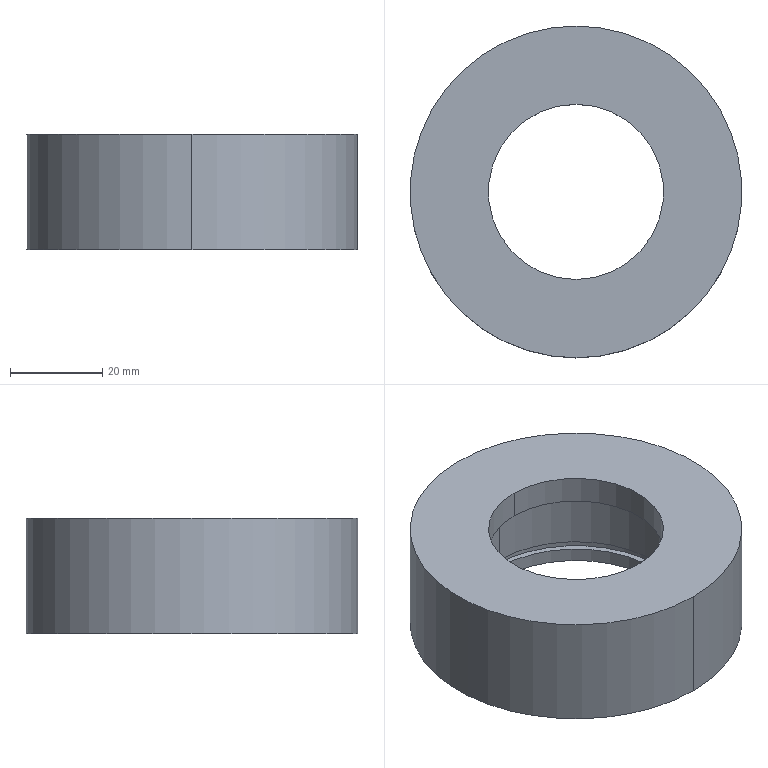Part | STEP file | DCV-000-003 | 1 solid | 15 faces | box 72 x 72 x 25 mm | volume 61649 mm3 | cylinder 10 | plane 5 | commonest cylinder face diameters 47 x4 38 x2 49.5 x2 72 x2
STEP:
#1=CARTESIAN_POINT('',(0.,0.,0.));
#2=DIRECTION('',(0.,0.,1.));
#3=DIRECTION('',(1.,0.,0.));
#4=AXIS2_PLACEMENT_3D('',#1,#2,#3);
#5=CARTESIAN_POINT('',(0.,19.,-6.));
#6=VERTEX_POINT('',#5);
#7=CARTESIAN_POINT('',(0.,19.,0.));
#8=VERTEX_POINT('',#7);
#9=CARTESIAN_POINT('',(0.,19.,-3.));
#10=DIRECTION('',(0.,0.,1.));
#11=VECTOR('',#10,1.);
#12=LINE('',#9,#11);
#13=CARTESIAN_POINT('',(0.,0.,-3.));
#14=DIRECTION('',(0.,0.,1.));
#15=DIRECTION('',(0.,1.,0.));
#16=AXIS2_PLACEMENT_3D('',#13,#14,#15);
#17=CYLINDRICAL_SURFACE('',#16,19.);
#18=CARTESIAN_POINT('',(6.283,0.));
#19=DIRECTION('',(0.,1.));
#20=VECTOR('',#19,1.);
#21=LINE('',#18,#20);
#22=(GEOMETRIC_REPRESENTATION_CONTEXT(2)PARAMETRIC_REPRESENTATION_CONTEXT()REPRESENTATION_CONTEXT('',''));
#23=DEFINITIONAL_REPRESENTATION('',(#21),#22);
#24=PCURVE('',#17,#23);
#25=CARTESIAN_POINT('',(0.,0.,-3.));
#26=DIRECTION('',(0.,0.,1.));
#27=DIRECTION('',(0.,1.,0.));
#28=AXIS2_PLACEMENT_3D('',#25,#26,#27);
#29=CYLINDRICAL_SURFACE('',#28,19.);
#30=CARTESIAN_POINT('',(0.,0.));
#31=DIRECTION('',(0.,1.));
#32=VECTOR('',#31,1.);
#33=LINE('',#30,#32);
#34=(GEOMETRIC_REPRESENTATION_CONTEXT(2)PARAMETRIC_REPRESENTATION_CONTEXT()REPRESENTATION_CONTEXT('',''));
#35=DEFINITIONAL_REPRESENTATION('',(#33),#34);
#36=PCURVE('',#29,#35);
#37=SURFACE_CURVE('',#12,(#24,#36),.PCURVE_S1.);
#38=EDGE_CURVE('',#6,#8,#37,.T.);
#39=ORIENTED_EDGE('',*,*,#38,.T.);
#40=CARTESIAN_POINT('',(0.,-19.,0.));
#41=VERTEX_POINT('',#40);
#42=CARTESIAN_POINT('',(0.,0.,0.));
#43=DIRECTION('',(0.,0.,1.));
#44=DIRECTION('',(1.,0.,0.));
#45=AXIS2_PLACEMENT_3D('',#42,#43,#44);
#46=CIRCLE('',#45,19.);
#47=CARTESIAN_POINT('',(-1.571,3.));
#48=DIRECTION('',(1.,0.));
#49=VECTOR('',#48,1.);
#50=LINE('',#47,#49);
#51=(GEOMETRIC_REPRESENTATION_CONTEXT(2)PARAMETRIC_REPRESENTATION_CONTEXT()REPRESENTATION_CONTEXT('',''));
#52=DEFINITIONAL_REPRESENTATION('',(#50),#51);
#53=PCURVE('',#17,#52);
#54=CARTESIAN_POINT('',(0.,19.,0.));
#55=DIRECTION('',(0.,0.,1.));
#56=DIRECTION('',(0.,-1.,0.));
#57=AXIS2_PLACEMENT_3D('',#54,#55,#56);
#58=PLANE('',#57);
#59=CARTESIAN_POINT('',(19.,0.));
#60=DIRECTION('',(0.,1.));
#61=AXIS2_PLACEMENT_2D('',#59,#60);
#62=CIRCLE('',#61,19.);
#63=(GEOMETRIC_REPRESENTATION_CONTEXT(2)PARAMETRIC_REPRESENTATION_CONTEXT()REPRESENTATION_CONTEXT('',''));
#64=DEFINITIONAL_REPRESENTATION('',(#62),#63);
#65=PCURVE('',#58,#64);
#66=SURFACE_CURVE('',#46,(#53,#65),.PCURVE_S1.);
#67=EDGE_CURVE('',#41,#8,#66,.T.);
#68=ORIENTED_EDGE('',*,*,#67,.F.);
#69=CARTESIAN_POINT('',(0.,-19.,-6.));
#70=VERTEX_POINT('',#69);
#71=CARTESIAN_POINT('',(0.,-19.,-3.));
#72=DIRECTION('',(0.,0.,1.));
#73=VECTOR('',#72,1.);
#74=LINE('',#71,#73);
#75=CARTESIAN_POINT('',(3.142,0.));
#76=DIRECTION('',(0.,1.));
#77=VECTOR('',#76,1.);
#78=LINE('',#75,#77);
#79=(GEOMETRIC_REPRESENTATION_CONTEXT(2)PARAMETRIC_REPRESENTATION_CONTEXT()REPRESENTATION_CONTEXT('',''));
#80=DEFINITIONAL_REPRESENTATION('',(#78),#79);
#81=PCURVE('',#17,#80);
#82=CARTESIAN_POINT('',(3.142,0.));
#83=DIRECTION('',(0.,1.));
#84=VECTOR('',#83,1.);
#85=LINE('',#82,#84);
#86=(GEOMETRIC_REPRESENTATION_CONTEXT(2)PARAMETRIC_REPRESENTATION_CONTEXT()REPRESENTATION_CONTEXT('',''));
#87=DEFINITIONAL_REPRESENTATION('',(#85),#86);
#88=PCURVE('',#29,#87);
#89=SURFACE_CURVE('',#74,(#81,#88),.PCURVE_S1.);
#90=EDGE_CURVE('',#70,#41,#89,.T.);
#91=ORIENTED_EDGE('',*,*,#90,.F.);
#92=CARTESIAN_POINT('',(0.,0.,-6.));
#93=DIRECTION('',(0.,0.,1.));
#94=DIRECTION('',(1.,0.,0.));
#95=AXIS2_PLACEMENT_3D('',#92,#93,#94);
#96=CIRCLE('',#95,19.);
#97=CARTESIAN_POINT('',(-1.571,-3.));
#98=DIRECTION('',(1.,0.));
#99=VECTOR('',#98,1.);
#100=LINE('',#97,#99);
#101=(GEOMETRIC_REPRESENTATION_CONTEXT(2)PARAMETRIC_REPRESENTATION_CONTEXT()REPRESENTATION_CONTEXT('',''));
#102=DEFINITIONAL_REPRESENTATION('',(#100),#101);
#103=PCURVE('',#17,#102);
#104=CARTESIAN_POINT('',(0.,23.5,-6.));
#105=DIRECTION('',(0.,0.,-1.));
#106=DIRECTION('',(-1.,0.,0.));
#107=AXIS2_PLACEMENT_3D('',#104,#105,#106);
#108=PLANE('',#107);
#109=CARTESIAN_POINT('',(-19.,-23.5));
#110=CARTESIAN_POINT('',(-19.,9.409));
#111=CARTESIAN_POINT('',(9.5,-7.046));
#112=CARTESIAN_POINT('',(38.,-23.5));
#113=CARTESIAN_POINT('',(9.5,-39.954));
#114=CARTESIAN_POINT('',(-19.,-56.409));
#115=CARTESIAN_POINT('',(-19.,-23.5));
#116=(BOUNDED_CURVE()B_SPLINE_CURVE(2,(#109,#110,#111,#112,#113,#114,#115),.UNSPECIFIED.,.T.,.F.)B_SPLINE_CURVE_WITH_KNOTS((1,2,2,2,2,1),(-2.094,0.,2.094,4.189,6.283,8.378),.UNSPECIFIED.)CURVE()GEOMETRIC_REPRESENTATION_ITEM()RATIONAL_B_SPLINE_CURVE((1.,0.5,1.,0.5,1.,0.5,1.))REPRESENTATION_ITEM(''));
#117=(GEOMETRIC_REPRESENTATION_CONTEXT(2)PARAMETRIC_REPRESENTATION_CONTEXT()REPRESENTATION_CONTEXT('',''));
#118=DEFINITIONAL_REPRESENTATION('',(#116),#117);
#119=PCURVE('',#108,#118);
#120=SURFACE_CURVE('',#96,(#103,#119),.PCURVE_S1.);
#121=EDGE_CURVE('',#70,#6,#120,.T.);
#122=ORIENTED_EDGE('',*,*,#121,.T.);
#123=EDGE_LOOP('',(#39,#68,#91,#122));
#124=FACE_BOUND('',#123,.F.);
#125=ADVANCED_FACE('',(#124),#17,.F.);
#126=CARTESIAN_POINT('',(0.,23.5,-20.));
#127=VERTEX_POINT('',#126);
#128=CARTESIAN_POINT('',(0.,23.5,-6.));
#129=VERTEX_POINT('',#128);
#130=CARTESIAN_POINT('',(0.,23.5,-13.));
#131=DIRECTION('',(0.,0.,1.));
#132=VECTOR('',#131,1.);
#133=LINE('',#130,#132);
#134=CARTESIAN_POINT('',(0.,0.,-13.));
#135=DIRECTION('',(0.,0.,1.));
#136=DIRECTION('',(0.,1.,0.));
#137=AXIS2_PLACEMENT_3D('',#134,#135,#136);
#138=CYLINDRICAL_SURFACE('',#137,23.5);
#139=CARTESIAN_POINT('',(6.283,0.));
#140=DIRECTION('',(0.,1.));
#141=VECTOR('',#140,1.);
#142=LINE('',#139,#141);
#143=(GEOMETRIC_REPRESENTATION_CONTEXT(2)PARAMETRIC_REPRESENTATION_CONTEXT()REPRESENTATION_CONTEXT('',''));
#144=DEFINITIONAL_REPRESENTATION('',(#142),#143);
#145=PCURVE('',#138,#144);
#146=CARTESIAN_POINT('',(0.,0.,-13.));
#147=DIRECTION('',(0.,0.,1.));
#148=DIRECTION('',(0.,1.,0.));
#149=AXIS2_PLACEMENT_3D('',#146,#147,#148);
#150=CYLINDRICAL_SURFACE('',#149,23.5);
#151=CARTESIAN_POINT('',(0.,0.));
#152=DIRECTION('',(0.,1.));
#153=VECTOR('',#152,1.);
#154=LINE('',#151,#153);
#155=(GEOMETRIC_REPRESENTATION_CONTEXT(2)PARAMETRIC_REPRESENTATION_CONTEXT()REPRESENTATION_CONTEXT('',''));
#156=DEFINITIONAL_REPRESENTATION('',(#154),#155);
#157=PCURVE('',#150,#156);
#158=SURFACE_CURVE('',#133,(#145,#157),.PCURVE_S1.);
#159=EDGE_CURVE('',#127,#129,#158,.T.);
#160=ORIENTED_EDGE('',*,*,#159,.T.);
#161=CARTESIAN_POINT('',(0.,-23.5,-6.));
#162=VERTEX_POINT('',#161);
#163=CARTESIAN_POINT('',(0.,0.,-6.));
#164=DIRECTION('',(0.,0.,1.));
#165=DIRECTION('',(1.,0.,0.));
#166=AXIS2_PLACEMENT_3D('',#163,#164,#165);
#167=CIRCLE('',#166,23.5);
#168=CARTESIAN_POINT('',(-1.571,7.));
#169=DIRECTION('',(1.,0.));
#170=VECTOR('',#169,1.);
#171=LINE('',#168,#170);
#172=(GEOMETRIC_REPRESENTATION_CONTEXT(2)PARAMETRIC_REPRESENTATION_CONTEXT()REPRESENTATION_CONTEXT('',''));
#173=DEFINITIONAL_REPRESENTATION('',(#171),#172);
#174=PCURVE('',#138,#173);
#175=CARTESIAN_POINT('',(-23.5,-23.5));
#176=CARTESIAN_POINT('',(-23.5,17.203));
#177=CARTESIAN_POINT('',(11.75,-3.148));
#178=CARTESIAN_POINT('',(47.,-23.5));
#179=CARTESIAN_POINT('',(11.75,-43.852));
#180=CARTESIAN_POINT('',(-23.5,-64.203));
#181=CARTESIAN_POINT('',(-23.5,-23.5));
#182=(BOUNDED_CURVE()B_SPLINE_CURVE(2,(#175,#176,#177,#178,#179,#180,#181),.UNSPECIFIED.,.T.,.F.)B_SPLINE_CURVE_WITH_KNOTS((1,2,2,2,2,1),(-2.094,0.,2.094,4.189,6.283,8.378),.UNSPECIFIED.)CURVE()GEOMETRIC_REPRESENTATION_ITEM()RATIONAL_B_SPLINE_CURVE((1.,0.5,1.,0.5,1.,0.5,1.))REPRESENTATION_ITEM(''));
#183=(GEOMETRIC_REPRESENTATION_CONTEXT(2)PARAMETRIC_REPRESENTATION_CONTEXT()REPRESENTATION_CONTEXT('',''));
#184=DEFINITIONAL_REPRESENTATION('',(#182),#183);
#185=PCURVE('',#108,#184);
#186=SURFACE_CURVE('',#167,(#174,#185),.PCURVE_S1.);
#187=EDGE_CURVE('',#162,#129,#186,.T.);
#188=ORIENTED_EDGE('',*,*,#187,.F.);
#189=CARTESIAN_POINT('',(0.,-23.5,-20.));
#190=VERTEX_POINT('',#189);
#191=CARTESIAN_POINT('',(0.,-23.5,-13.));
#192=DIRECTION('',(0.,0.,1.));
#193=VECTOR('',#192,1.);
#194=LINE('',#191,#193);
#195=CARTESIAN_POINT('',(3.142,0.));
#196=DIRECTION('',(0.,1.));
#197=VECTOR('',#196,1.);
#198=LINE('',#195,#197);
#199=(GEOMETRIC_REPRESENTATION_CONTEXT(2)PARAMETRIC_REPRESENTATION_CONTEXT()REPRESENTATION_CONTEXT('',''));
#200=DEFINITIONAL_REPRESENTATION('',(#198),#199);
#201=PCURVE('',#138,#200);
#202=CARTESIAN_POINT('',(3.142,0.));
#203=DIRECTION('',(0.,1.));
#204=VECTOR('',#203,1.);
#205=LINE('',#202,#204);
#206=(GEOMETRIC_REPRESENTATION_CONTEXT(2)PARAMETRIC_REPRESENTATION_CONTEXT()REPRESENTATION_CONTEXT('',''));
#207=DEFINITIONAL_REPRESENTATION('',(#205),#206);
#208=PCURVE('',#150,#207);
#209=SURFACE_CURVE('',#194,(#201,#208),.PCURVE_S1.);
#210=EDGE_CURVE('',#190,#162,#209,.T.);
#211=ORIENTED_EDGE('',*,*,#210,.F.);
#212=CARTESIAN_POINT('',(0.,0.,-20.));
#213=DIRECTION('',(0.,0.,1.));
#214=DIRECTION('',(1.,0.,0.));
#215=AXIS2_PLACEMENT_3D('',#212,#213,#214);
#216=CIRCLE('',#215,23.5);
#217=CARTESIAN_POINT('',(-1.571,-7.));
#218=DIRECTION('',(1.,0.));
#219=VECTOR('',#218,1.);
#220=LINE('',#217,#219);
#221=(GEOMETRIC_REPRESENTATION_CONTEXT(2)PARAMETRIC_REPRESENTATION_CONTEXT()REPRESENTATION_CONTEXT('',''));
#222=DEFINITIONAL_REPRESENTATION('',(#220),#221);
#223=PCURVE('',#138,#222);
#224=CARTESIAN_POINT('',(0.,24.75,-20.));
#225=DIRECTION('',(0.,0.,-1.));
#226=DIRECTION('',(-1.,0.,0.));
#227=AXIS2_PLACEMENT_3D('',#224,#225,#226);
#228=PLANE('',#227);
#229=CARTESIAN_POINT('',(-23.5,-24.75));
#230=CARTESIAN_POINT('',(-23.5,15.953));
#231=CARTESIAN_POINT('',(11.75,-4.398));
#232=CARTESIAN_POINT('',(47.,-24.75));
#233=CARTESIAN_POINT('',(11.75,-45.102));
#234=CARTESIAN_POINT('',(-23.5,-65.453));
#235=CARTESIAN_POINT('',(-23.5,-24.75));
#236=(BOUNDED_CURVE()B_SPLINE_CURVE(2,(#229,#230,#231,#232,#233,#234,#235),.UNSPECIFIED.,.T.,.F.)B_SPLINE_CURVE_WITH_KNOTS((1,2,2,2,2,1),(-2.094,0.,2.094,4.189,6.283,8.378),.UNSPECIFIED.)CURVE()GEOMETRIC_REPRESENTATION_ITEM()RATIONAL_B_SPLINE_CURVE((1.,0.5,1.,0.5,1.,0.5,1.))REPRESENTATION_ITEM(''));
#237=(GEOMETRIC_REPRESENTATION_CONTEXT(2)PARAMETRIC_REPRESENTATION_CONTEXT()REPRESENTATION_CONTEXT('',''));
#238=DEFINITIONAL_REPRESENTATION('',(#236),#237);
#239=PCURVE('',#228,#238);
#240=SURFACE_CURVE('',#216,(#223,#239),.PCURVE_S1.);
#241=EDGE_CURVE('',#190,#127,#240,.T.);
#242=ORIENTED_EDGE('',*,*,#241,.T.);
#243=EDGE_LOOP('',(#160,#188,#211,#242));
#244=FACE_BOUND('',#243,.F.);
#245=ADVANCED_FACE('',(#244),#138,.F.);
#246=CARTESIAN_POINT('',(0.,24.75,-21.95));
#247=VERTEX_POINT('',#246);
#248=CARTESIAN_POINT('',(0.,24.75,-20.));
#249=VERTEX_POINT('',#248);
#250=CARTESIAN_POINT('',(0.,24.75,-20.975));
#251=DIRECTION('',(0.,0.,1.));
#252=VECTOR('',#251,1.);
#253=LINE('',#250,#252);
#254=CARTESIAN_POINT('',(0.,0.,-20.975));
#255=DIRECTION('',(0.,0.,1.));
#256=DIRECTION('',(0.,1.,0.));
#257=AXIS2_PLACEMENT_3D('',#254,#255,#256);
#258=CYLINDRICAL_SURFACE('',#257,24.75);
#259=CARTESIAN_POINT('',(6.283,0.));
#260=DIRECTION('',(0.,1.));
#261=VECTOR('',#260,1.);
#262=LINE('',#259,#261);
#263=(GEOMETRIC_REPRESENTATION_CONTEXT(2)PARAMETRIC_REPRESENTATION_CONTEXT()REPRESENTATION_CONTEXT('',''));
#264=DEFINITIONAL_REPRESENTATION('',(#262),#263);
#265=PCURVE('',#258,#264);
#266=CARTESIAN_POINT('',(0.,0.,-20.975));
#267=DIRECTION('',(0.,0.,1.));
#268=DIRECTION('',(0.,1.,0.));
#269=AXIS2_PLACEMENT_3D('',#266,#267,#268);
#270=CYLINDRICAL_SURFACE('',#269,24.75);
#271=CARTESIAN_POINT('',(0.,0.));
#272=DIRECTION('',(0.,1.));
#273=VECTOR('',#272,1.);
#274=LINE('',#271,#273);
#275=(GEOMETRIC_REPRESENTATION_CONTEXT(2)PARAMETRIC_REPRESENTATION_CONTEXT()REPRESENTATION_CONTEXT('',''));
#276=DEFINITIONAL_REPRESENTATION('',(#274),#275);
#277=PCURVE('',#270,#276);
#278=SURFACE_CURVE('',#253,(#265,#277),.PCURVE_S1.);
#279=EDGE_CURVE('',#247,#249,#278,.T.);
#280=ORIENTED_EDGE('',*,*,#279,.T.);
#281=CARTESIAN_POINT('',(0.,-24.75,-20.));
#282=VERTEX_POINT('',#281);
#283=CARTESIAN_POINT('',(0.,0.,-20.));
#284=DIRECTION('',(0.,0.,1.));
#285=DIRECTION('',(1.,0.,0.));
#286=AXIS2_PLACEMENT_3D('',#283,#284,#285);
#287=CIRCLE('',#286,24.75);
#288=CARTESIAN_POINT('',(-1.571,0.975));
#289=DIRECTION('',(1.,0.));
#290=VECTOR('',#289,1.);
#291=LINE('',#288,#290);
#292=(GEOMETRIC_REPRESENTATION_CONTEXT(2)PARAMETRIC_REPRESENTATION_CONTEXT()REPRESENTATION_CONTEXT('',''));
#293=DEFINITIONAL_REPRESENTATION('',(#291),#292);
#294=PCURVE('',#258,#293);
#295=CARTESIAN_POINT('',(-24.75,-24.75));
#296=CARTESIAN_POINT('',(-24.75,18.118));
#297=CARTESIAN_POINT('',(12.375,-3.316));
#298=CARTESIAN_POINT('',(49.5,-24.75));
#299=CARTESIAN_POINT('',(12.375,-46.184));
#300=CARTESIAN_POINT('',(-24.75,-67.618));
#301=CARTESIAN_POINT('',(-24.75,-24.75));
#302=(BOUNDED_CURVE()B_SPLINE_CURVE(2,(#295,#296,#297,#298,#299,#300,#301),.UNSPECIFIED.,.T.,.F.)B_SPLINE_CURVE_WITH_KNOTS((1,2,2,2,2,1),(-2.094,0.,2.094,4.189,6.283,8.378),.UNSPECIFIED.)CURVE()GEOMETRIC_REPRESENTATION_ITEM()RATIONAL_B_SPLINE_CURVE((1.,0.5,1.,0.5,1.,0.5,1.))REPRESENTATION_ITEM(''));
#303=(GEOMETRIC_REPRESENTATION_CONTEXT(2)PARAMETRIC_REPRESENTATION_CONTEXT()REPRESENTATION_CONTEXT('',''));
#304=DEFINITIONAL_REPRESENTATION('',(#302),#303);
#305=PCURVE('',#228,#304);
#306=SURFACE_CURVE('',#287,(#294,#305),.PCURVE_S1.);
#307=EDGE_CURVE('',#282,#249,#306,.T.);
#308=ORIENTED_EDGE('',*,*,#307,.F.);
#309=CARTESIAN_POINT('',(0.,-24.75,-21.95));
#310=VERTEX_POINT('',#309);
#311=CARTESIAN_POINT('',(0.,-24.75,-20.975));
#312=DIRECTION('',(0.,0.,1.));
#313=VECTOR('',#312,1.);
#314=LINE('',#311,#313);
#315=CARTESIAN_POINT('',(3.142,0.));
#316=DIRECTION('',(0.,1.));
#317=VECTOR('',#316,1.);
#318=LINE('',#315,#317);
#319=(GEOMETRIC_REPRESENTATION_CONTEXT(2)PARAMETRIC_REPRESENTATION_CONTEXT()REPRESENTATION_CONTEXT('',''));
#320=DEFINITIONAL_REPRESENTATION('',(#318),#319);
#321=PCURVE('',#258,#320);
#322=CARTESIAN_POINT('',(3.142,0.));
#323=DIRECTION('',(0.,1.));
#324=VECTOR('',#323,1.);
#325=LINE('',#322,#324);
#326=(GEOMETRIC_REPRESENTATION_CONTEXT(2)PARAMETRIC_REPRESENTATION_CONTEXT()REPRESENTATION_CONTEXT('',''));
#327=DEFINITIONAL_REPRESENTATION('',(#325),#326);
#328=PCURVE('',#270,#327);
#329=SURFACE_CURVE('',#314,(#321,#328),.PCURVE_S1.);
#330=EDGE_CURVE('',#310,#282,#329,.T.);
#331=ORIENTED_EDGE('',*,*,#330,.F.);
#332=CARTESIAN_POINT('',(0.,0.,-21.95));
#333=DIRECTION('',(0.,0.,1.));
#334=DIRECTION('',(1.,0.,0.));
#335=AXIS2_PLACEMENT_3D('',#332,#333,#334);
#336=CIRCLE('',#335,24.75);
#337=CARTESIAN_POINT('',(-1.571,-0.975));
#338=DIRECTION('',(1.,0.));
#339=VECTOR('',#338,1.);
#340=LINE('',#337,#339);
#341=(GEOMETRIC_REPRESENTATION_CONTEXT(2)PARAMETRIC_REPRESENTATION_CONTEXT()REPRESENTATION_CONTEXT('',''));
#342=DEFINITIONAL_REPRESENTATION('',(#340),#341);
#343=PCURVE('',#258,#342);
#344=CARTESIAN_POINT('',(0.,23.5,-21.95));
#345=DIRECTION('',(0.,0.,1.));
#346=DIRECTION('',(0.,-1.,0.));
#347=AXIS2_PLACEMENT_3D('',#344,#345,#346);
#348=PLANE('',#347);
#349=CARTESIAN_POINT('',(23.5,0.));
#350=DIRECTION('',(0.,1.));
#351=AXIS2_PLACEMENT_2D('',#349,#350);
#352=CIRCLE('',#351,24.75);
#353=(GEOMETRIC_REPRESENTATION_CONTEXT(2)PARAMETRIC_REPRESENTATION_CONTEXT()REPRESENTATION_CONTEXT('',''));
#354=DEFINITIONAL_REPRESENTATION('',(#352),#353);
#355=PCURVE('',#348,#354);
#356=SURFACE_CURVE('',#336,(#343,#355),.PCURVE_S1.);
#357=EDGE_CURVE('',#310,#247,#356,.T.);
#358=ORIENTED_EDGE('',*,*,#357,.T.);
#359=EDGE_LOOP('',(#280,#308,#331,#358));
#360=FACE_BOUND('',#359,.F.);
#361=ADVANCED_FACE('',(#360),#258,.F.);
#362=CARTESIAN_POINT('',(0.,23.5,-25.));
#363=VERTEX_POINT('',#362);
#364=CARTESIAN_POINT('',(0.,23.5,-21.95));
#365=VERTEX_POINT('',#364);
#366=CARTESIAN_POINT('',(0.,23.5,-23.475));
#367=DIRECTION('',(0.,0.,1.));
#368=VECTOR('',#367,1.);
#369=LINE('',#366,#368);
#370=CARTESIAN_POINT('',(0.,0.,-23.475));
#371=DIRECTION('',(0.,0.,1.));
#372=DIRECTION('',(0.,1.,0.));
#373=AXIS2_PLACEMENT_3D('',#370,#371,#372);
#374=CYLINDRICAL_SURFACE('',#373,23.5);
#375=CARTESIAN_POINT('',(6.283,0.));
#376=DIRECTION('',(0.,1.));
#377=VECTOR('',#376,1.);
#378=LINE('',#375,#377);
#379=(GEOMETRIC_REPRESENTATION_CONTEXT(2)PARAMETRIC_REPRESENTATION_CONTEXT()REPRESENTATION_CONTEXT('',''));
#380=DEFINITIONAL_REPRESENTATION('',(#378),#379);
#381=PCURVE('',#374,#380);
#382=CARTESIAN_POINT('',(0.,0.,-23.475));
#383=DIRECTION('',(0.,0.,1.));
#384=DIRECTION('',(0.,1.,0.));
#385=AXIS2_PLACEMENT_3D('',#382,#383,#384);
#386=CYLINDRICAL_SURFACE('',#385,23.5);
#387=CARTESIAN_POINT('',(0.,0.));
#388=DIRECTION('',(0.,1.));
#389=VECTOR('',#388,1.);
#390=LINE('',#387,#389);
#391=(GEOMETRIC_REPRESENTATION_CONTEXT(2)PARAMETRIC_REPRESENTATION_CONTEXT()REPRESENTATION_CONTEXT('',''));
#392=DEFINITIONAL_REPRESENTATION('',(#390),#391);
#393=PCURVE('',#386,#392);
#394=SURFACE_CURVE('',#369,(#381,#393),.PCURVE_S1.);
#395=EDGE_CURVE('',#363,#365,#394,.T.);
#396=ORIENTED_EDGE('',*,*,#395,.T.);
#397=CARTESIAN_POINT('',(0.,-23.5,-21.95));
#398=VERTEX_POINT('',#397);
#399=CARTESIAN_POINT('',(0.,0.,-21.95));
#400=DIRECTION('',(0.,0.,1.));
#401=DIRECTION('',(1.,0.,0.));
#402=AXIS2_PLACEMENT_3D('',#399,#400,#401);
#403=CIRCLE('',#402,23.5);
#404=CARTESIAN_POINT('',(-1.571,1.525));
#405=DIRECTION('',(1.,0.));
#406=VECTOR('',#405,1.);
#407=LINE('',#404,#406);
#408=(GEOMETRIC_REPRESENTATION_CONTEXT(2)PARAMETRIC_REPRESENTATION_CONTEXT()REPRESENTATION_CONTEXT('',''));
#409=DEFINITIONAL_REPRESENTATION('',(#407),#408);
#410=PCURVE('',#374,#409);
#411=CARTESIAN_POINT('',(23.5,0.));
#412=DIRECTION('',(0.,1.));
#413=AXIS2_PLACEMENT_2D('',#411,#412);
#414=CIRCLE('',#413,23.5);
#415=(GEOMETRIC_REPRESENTATION_CONTEXT(2)PARAMETRIC_REPRESENTATION_CONTEXT()REPRESENTATION_CONTEXT('',''));
#416=DEFINITIONAL_REPRESENTATION('',(#414),#415);
#417=PCURVE('',#348,#416);
#418=SURFACE_CURVE('',#403,(#410,#417),.PCURVE_S1.);
#419=EDGE_CURVE('',#398,#365,#418,.T.);
#420=ORIENTED_EDGE('',*,*,#419,.F.);
#421=CARTESIAN_POINT('',(0.,-23.5,-25.));
#422=VERTEX_POINT('',#421);
#423=CARTESIAN_POINT('',(0.,-23.5,-23.475));
#424=DIRECTION('',(0.,0.,1.));
#425=VECTOR('',#424,1.);
#426=LINE('',#423,#425);
#427=CARTESIAN_POINT('',(3.142,0.));
#428=DIRECTION('',(0.,1.));
#429=VECTOR('',#428,1.);
#430=LINE('',#427,#429);
#431=(GEOMETRIC_REPRESENTATION_CONTEXT(2)PARAMETRIC_REPRESENTATION_CONTEXT()REPRESENTATION_CONTEXT('',''));
#432=DEFINITIONAL_REPRESENTATION('',(#430),#431);
#433=PCURVE('',#374,#432);
#434=CARTESIAN_POINT('',(3.142,0.));
#435=DIRECTION('',(0.,1.));
#436=VECTOR('',#435,1.);
#437=LINE('',#434,#436);
#438=(GEOMETRIC_REPRESENTATION_CONTEXT(2)PARAMETRIC_REPRESENTATION_CONTEXT()REPRESENTATION_CONTEXT('',''));
#439=DEFINITIONAL_REPRESENTATION('',(#437),#438);
#440=PCURVE('',#386,#439);
#441=SURFACE_CURVE('',#426,(#433,#440),.PCURVE_S1.);
#442=EDGE_CURVE('',#422,#398,#441,.T.);
#443=ORIENTED_EDGE('',*,*,#442,.F.);
#444=CARTESIAN_POINT('',(0.,0.,-25.));
#445=DIRECTION('',(0.,0.,1.));
#446=DIRECTION('',(1.,0.,0.));
#447=AXIS2_PLACEMENT_3D('',#444,#445,#446);
#448=CIRCLE('',#447,23.5);
#449=CARTESIAN_POINT('',(-1.571,-1.525));
#450=DIRECTION('',(1.,0.));
#451=VECTOR('',#450,1.);
#452=LINE('',#449,#451);
#453=(GEOMETRIC_REPRESENTATION_CONTEXT(2)PARAMETRIC_REPRESENTATION_CONTEXT()REPRESENTATION_CONTEXT('',''));
#454=DEFINITIONAL_REPRESENTATION('',(#452),#453);
#455=PCURVE('',#374,#454);
#456=CARTESIAN_POINT('',(0.,36.,-25.));
#457=DIRECTION('',(0.,0.,-1.));
#458=DIRECTION('',(-1.,0.,0.));
#459=AXIS2_PLACEMENT_3D('',#456,#457,#458);
#460=PLANE('',#459);
#461=CARTESIAN_POINT('',(-23.5,-36.));
#462=CARTESIAN_POINT('',(-23.5,4.703));
#463=CARTESIAN_POINT('',(11.75,-15.648));
#464=CARTESIAN_POINT('',(47.,-36.));
#465=CARTESIAN_POINT('',(11.75,-56.352));
#466=CARTESIAN_POINT('',(-23.5,-76.703));
#467=CARTESIAN_POINT('',(-23.5,-36.));
#468=(BOUNDED_CURVE()B_SPLINE_CURVE(2,(#461,#462,#463,#464,#465,#466,#467),.UNSPECIFIED.,.T.,.F.)B_SPLINE_CURVE_WITH_KNOTS((1,2,2,2,2,1),(-2.094,0.,2.094,4.189,6.283,8.378),.UNSPECIFIED.)CURVE()GEOMETRIC_REPRESENTATION_ITEM()RATIONAL_B_SPLINE_CURVE((1.,0.5,1.,0.5,1.,0.5,1.))REPRESENTATION_ITEM(''));
#469=(GEOMETRIC_REPRESENTATION_CONTEXT(2)PARAMETRIC_REPRESENTATION_CONTEXT()REPRESENTATION_CONTEXT('',''));
#470=DEFINITIONAL_REPRESENTATION('',(#468),#469);
#471=PCURVE('',#460,#470);
#472=SURFACE_CURVE('',#448,(#455,#471),.PCURVE_S1.);
#473=EDGE_CURVE('',#422,#363,#472,.T.);
#474=ORIENTED_EDGE('',*,*,#473,.T.);
#475=EDGE_LOOP('',(#396,#420,#443,#474));
#476=FACE_BOUND('',#475,.F.);
#477=ADVANCED_FACE('',(#476),#374,.F.);
#478=CARTESIAN_POINT('',(0.,36.,-25.));
#479=VERTEX_POINT('',#478);
#480=CARTESIAN_POINT('',(0.,-36.,-25.));
#481=VERTEX_POINT('',#480);
#482=CARTESIAN_POINT('',(0.,0.,-25.));
#483=DIRECTION('',(0.,0.,1.));
#484=DIRECTION('',(1.,0.,0.));
#485=AXIS2_PLACEMENT_3D('',#482,#483,#484);
#486=CIRCLE('',#485,36.);
#487=CARTESIAN_POINT('',(0.,0.,-12.5));
#488=DIRECTION('',(0.,0.,1.));
#489=DIRECTION('',(0.,1.,0.));
#490=AXIS2_PLACEMENT_3D('',#487,#488,#489);
#491=CYLINDRICAL_SURFACE('',#490,36.);
#492=CARTESIAN_POINT('',(-1.571,-12.5));
#493=DIRECTION('',(1.,0.));
#494=VECTOR('',#493,1.);
#495=LINE('',#492,#494);
#496=(GEOMETRIC_REPRESENTATION_CONTEXT(2)PARAMETRIC_REPRESENTATION_CONTEXT()REPRESENTATION_CONTEXT('',''));
#497=DEFINITIONAL_REPRESENTATION('',(#495),#496);
#498=PCURVE('',#491,#497);
#499=CARTESIAN_POINT('',(-36.,-36.));
#500=CARTESIAN_POINT('',(-36.,26.354));
#501=CARTESIAN_POINT('',(18.,-4.823));
#502=CARTESIAN_POINT('',(72.,-36.));
#503=CARTESIAN_POINT('',(18.,-67.177));
#504=CARTESIAN_POINT('',(-36.,-98.354));
#505=CARTESIAN_POINT('',(-36.,-36.));
#506=(BOUNDED_CURVE()B_SPLINE_CURVE(2,(#499,#500,#501,#502,#503,#504,#505),.UNSPECIFIED.,.T.,.F.)B_SPLINE_CURVE_WITH_KNOTS((1,2,2,2,2,1),(-2.094,0.,2.094,4.189,6.283,8.378),.UNSPECIFIED.)CURVE()GEOMETRIC_REPRESENTATION_ITEM()RATIONAL_B_SPLINE_CURVE((1.,0.5,1.,0.5,1.,0.5,1.))REPRESENTATION_ITEM(''));
#507=(GEOMETRIC_REPRESENTATION_CONTEXT(2)PARAMETRIC_REPRESENTATION_CONTEXT()REPRESENTATION_CONTEXT('',''));
#508=DEFINITIONAL_REPRESENTATION('',(#506),#507);
#509=PCURVE('',#460,#508);
#510=SURFACE_CURVE('',#486,(#498,#509),.PCURVE_S1.);
#511=EDGE_CURVE('',#479,#481,#510,.T.);
#512=ORIENTED_EDGE('',*,*,#511,.T.);
#513=CARTESIAN_POINT('',(0.,-36.,0.));
#514=VERTEX_POINT('',#513);
#515=CARTESIAN_POINT('',(0.,-36.,-12.5));
#516=DIRECTION('',(0.,0.,1.));
#517=VECTOR('',#516,1.);
#518=LINE('',#515,#517);
#519=CARTESIAN_POINT('',(3.142,0.));
#520=DIRECTION('',(0.,1.));
#521=VECTOR('',#520,1.);
#522=LINE('',#519,#521);
#523=(GEOMETRIC_REPRESENTATION_CONTEXT(2)PARAMETRIC_REPRESENTATION_CONTEXT()REPRESENTATION_CONTEXT('',''));
#524=DEFINITIONAL_REPRESENTATION('',(#522),#523);
#525=PCURVE('',#491,#524);
#526=CARTESIAN_POINT('',(0.,0.,-12.5));
#527=DIRECTION('',(0.,0.,1.));
#528=DIRECTION('',(0.,1.,0.));
#529=AXIS2_PLACEMENT_3D('',#526,#527,#528);
#530=CYLINDRICAL_SURFACE('',#529,36.);
#531=CARTESIAN_POINT('',(3.142,0.));
#532=DIRECTION('',(0.,1.));
#533=VECTOR('',#532,1.);
#534=LINE('',#531,#533);
#535=(GEOMETRIC_REPRESENTATION_CONTEXT(2)PARAMETRIC_REPRESENTATION_CONTEXT()REPRESENTATION_CONTEXT('',''));
#536=DEFINITIONAL_REPRESENTATION('',(#534),#535);
#537=PCURVE('',#530,#536);
#538=SURFACE_CURVE('',#518,(#525,#537),.PCURVE_S1.);
#539=EDGE_CURVE('',#481,#514,#538,.T.);
#540=ORIENTED_EDGE('',*,*,#539,.T.);
#541=CARTESIAN_POINT('',(0.,36.,0.));
#542=VERTEX_POINT('',#541);
#543=CARTESIAN_POINT('',(0.,0.,0.));
#544=DIRECTION('',(0.,0.,1.));
#545=DIRECTION('',(1.,0.,0.));
#546=AXIS2_PLACEMENT_3D('',#543,#544,#545);
#547=CIRCLE('',#546,36.);
#548=CARTESIAN_POINT('',(-1.571,12.5));
#549=DIRECTION('',(1.,0.));
#550=VECTOR('',#549,1.);
#551=LINE('',#548,#550);
#552=(GEOMETRIC_REPRESENTATION_CONTEXT(2)PARAMETRIC_REPRESENTATION_CONTEXT()REPRESENTATION_CONTEXT('',''));
#553=DEFINITIONAL_REPRESENTATION('',(#551),#552);
#554=PCURVE('',#491,#553);
#555=CARTESIAN_POINT('',(19.,0.));
#556=DIRECTION('',(0.,1.));
#557=AXIS2_PLACEMENT_2D('',#555,#556);
#558=CIRCLE('',#557,36.);
#559=(GEOMETRIC_REPRESENTATION_CONTEXT(2)PARAMETRIC_REPRESENTATION_CONTEXT()REPRESENTATION_CONTEXT('',''));
#560=DEFINITIONAL_REPRESENTATION('',(#558),#559);
#561=PCURVE('',#58,#560);
#562=SURFACE_CURVE('',#547,(#554,#561),.PCURVE_S1.);
#563=EDGE_CURVE('',#542,#514,#562,.T.);
#564=ORIENTED_EDGE('',*,*,#563,.F.);
#565=CARTESIAN_POINT('',(0.,36.,-12.5));
#566=DIRECTION('',(0.,0.,1.));
#567=VECTOR('',#566,1.);
#568=LINE('',#565,#567);
#569=CARTESIAN_POINT('',(0.,0.));
#570=DIRECTION('',(0.,1.));
#571=VECTOR('',#570,1.);
#572=LINE('',#569,#571);
#573=(GEOMETRIC_REPRESENTATION_CONTEXT(2)PARAMETRIC_REPRESENTATION_CONTEXT()REPRESENTATION_CONTEXT('',''));
#574=DEFINITIONAL_REPRESENTATION('',(#572),#573);
#575=PCURVE('',#491,#574);
#576=CARTESIAN_POINT('',(6.283,0.));
#577=DIRECTION('',(0.,1.));
#578=VECTOR('',#577,1.);
#579=LINE('',#576,#578);
#580=(GEOMETRIC_REPRESENTATION_CONTEXT(2)PARAMETRIC_REPRESENTATION_CONTEXT()REPRESENTATION_CONTEXT('',''));
#581=DEFINITIONAL_REPRESENTATION('',(#579),#580);
#582=PCURVE('',#530,#581);
#583=SURFACE_CURVE('',#568,(#575,#582),.PCURVE_S1.);
#584=EDGE_CURVE('',#479,#542,#583,.T.);
#585=ORIENTED_EDGE('',*,*,#584,.F.);
#586=EDGE_LOOP('',(#512,#540,#564,#585));
#587=FACE_BOUND('',#586,.T.);
#588=ADVANCED_FACE('',(#587),#491,.T.);
#589=ORIENTED_EDGE('',*,*,#539,.F.);
#590=CARTESIAN_POINT('',(0.,0.,-25.));
#591=DIRECTION('',(0.,0.,1.));
#592=DIRECTION('',(1.,0.,0.));
#593=AXIS2_PLACEMENT_3D('',#590,#591,#592);
#594=CIRCLE('',#593,36.);
#595=CARTESIAN_POINT('',(-1.571,-12.5));
#596=DIRECTION('',(1.,0.));
#597=VECTOR('',#596,1.);
#598=LINE('',#595,#597);
#599=(GEOMETRIC_REPRESENTATION_CONTEXT(2)PARAMETRIC_REPRESENTATION_CONTEXT()REPRESENTATION_CONTEXT('',''));
#600=DEFINITIONAL_REPRESENTATION('',(#598),#599);
#601=PCURVE('',#530,#600);
#602=CARTESIAN_POINT('',(-36.,-36.));
#603=CARTESIAN_POINT('',(-36.,26.354));
#604=CARTESIAN_POINT('',(18.,-4.823));
#605=CARTESIAN_POINT('',(72.,-36.));
#606=CARTESIAN_POINT('',(18.,-67.177));
#607=CARTESIAN_POINT('',(-36.,-98.354));
#608=CARTESIAN_POINT('',(-36.,-36.));
#609=(BOUNDED_CURVE()B_SPLINE_CURVE(2,(#602,#603,#604,#605,#606,#607,#608),.UNSPECIFIED.,.T.,.F.)B_SPLINE_CURVE_WITH_KNOTS((1,2,2,2,2,1),(-2.094,0.,2.094,4.189,6.283,8.378),.UNSPECIFIED.)CURVE()GEOMETRIC_REPRESENTATION_ITEM()RATIONAL_B_SPLINE_CURVE((1.,0.5,1.,0.5,1.,0.5,1.))REPRESENTATION_ITEM(''));
#610=(GEOMETRIC_REPRESENTATION_CONTEXT(2)PARAMETRIC_REPRESENTATION_CONTEXT()REPRESENTATION_CONTEXT('',''));
#611=DEFINITIONAL_REPRESENTATION('',(#609),#610);
#612=PCURVE('',#460,#611);
#613=SURFACE_CURVE('',#594,(#601,#612),.PCURVE_S1.);
#614=EDGE_CURVE('',#481,#479,#613,.T.);
#615=ORIENTED_EDGE('',*,*,#614,.T.);
#616=ORIENTED_EDGE('',*,*,#584,.T.);
#617=CARTESIAN_POINT('',(0.,0.,0.));
#618=DIRECTION('',(0.,0.,1.));
#619=DIRECTION('',(1.,0.,0.));
#620=AXIS2_PLACEMENT_3D('',#617,#618,#619);
#621=CIRCLE('',#620,36.);
#622=CARTESIAN_POINT('',(-1.571,12.5));
#623=DIRECTION('',(1.,0.));
#624=VECTOR('',#623,1.);
#625=LINE('',#622,#624);
#626=(GEOMETRIC_REPRESENTATION_CONTEXT(2)PARAMETRIC_REPRESENTATION_CONTEXT()REPRESENTATION_CONTEXT('',''));
#627=DEFINITIONAL_REPRESENTATION('',(#625),#626);
#628=PCURVE('',#530,#627);
#629=CARTESIAN_POINT('',(19.,0.));
#630=DIRECTION('',(0.,1.));
#631=AXIS2_PLACEMENT_2D('',#629,#630);
#632=CIRCLE('',#631,36.);
#633=(GEOMETRIC_REPRESENTATION_CONTEXT(2)PARAMETRIC_REPRESENTATION_CONTEXT()REPRESENTATION_CONTEXT('',''));
#634=DEFINITIONAL_REPRESENTATION('',(#632),#633);
#635=PCURVE('',#58,#634);
#636=SURFACE_CURVE('',#621,(#628,#635),.PCURVE_S1.);
#637=EDGE_CURVE('',#514,#542,#636,.T.);
#638=ORIENTED_EDGE('',*,*,#637,.F.);
#639=EDGE_LOOP('',(#589,#615,#616,#638));
#640=FACE_BOUND('',#639,.T.);
#641=ADVANCED_FACE('',(#640),#530,.T.);
#642=CARTESIAN_POINT('',(0.,0.,-25.));
#643=DIRECTION('',(0.,0.,1.));
#644=DIRECTION('',(1.,0.,0.));
#645=AXIS2_PLACEMENT_3D('',#642,#643,#644);
#646=CIRCLE('',#645,23.5);
#647=CARTESIAN_POINT('',(-23.5,-36.));
#648=CARTESIAN_POINT('',(-23.5,4.703));
#649=CARTESIAN_POINT('',(11.75,-15.648));
#650=CARTESIAN_POINT('',(47.,-36.));
#651=CARTESIAN_POINT('',(11.75,-56.352));
#652=CARTESIAN_POINT('',(-23.5,-76.703));
#653=CARTESIAN_POINT('',(-23.5,-36.));
#654=(BOUNDED_CURVE()B_SPLINE_CURVE(2,(#647,#648,#649,#650,#651,#652,#653),.UNSPECIFIED.,.T.,.F.)B_SPLINE_CURVE_WITH_KNOTS((1,2,2,2,2,1),(-2.094,0.,2.094,4.189,6.283,8.378),.UNSPECIFIED.)CURVE()GEOMETRIC_REPRESENTATION_ITEM()RATIONAL_B_SPLINE_CURVE((1.,0.5,1.,0.5,1.,0.5,1.))REPRESENTATION_ITEM(''));
#655=(GEOMETRIC_REPRESENTATION_CONTEXT(2)PARAMETRIC_REPRESENTATION_CONTEXT()REPRESENTATION_CONTEXT('',''));
#656=DEFINITIONAL_REPRESENTATION('',(#654),#655);
#657=PCURVE('',#460,#656);
#658=CARTESIAN_POINT('',(-1.571,-1.525));
#659=DIRECTION('',(1.,0.));
#660=VECTOR('',#659,1.);
#661=LINE('',#658,#660);
#662=(GEOMETRIC_REPRESENTATION_CONTEXT(2)PARAMETRIC_REPRESENTATION_CONTEXT()REPRESENTATION_CONTEXT('',''));
#663=DEFINITIONAL_REPRESENTATION('',(#661),#662);
#664=PCURVE('',#386,#663);
#665=SURFACE_CURVE('',#646,(#657,#664),.PCURVE_S1.);
#666=EDGE_CURVE('',#363,#422,#665,.T.);
#667=ORIENTED_EDGE('',*,*,#666,.T.);
#668=ORIENTED_EDGE('',*,*,#473,.T.);
#669=EDGE_LOOP('',(#667,#668));
#670=FACE_BOUND('',#669,.T.);
#671=ORIENTED_EDGE('',*,*,#511,.F.);
#672=ORIENTED_EDGE('',*,*,#614,.F.);
#673=EDGE_LOOP('',(#671,#672));
#674=FACE_BOUND('',#673,.T.);
#675=ADVANCED_FACE('',(#670,#674),#460,.T.);
#676=CARTESIAN_POINT('',(0.,0.,-21.95));
#677=DIRECTION('',(0.,0.,1.));
#678=DIRECTION('',(1.,0.,0.));
#679=AXIS2_PLACEMENT_3D('',#676,#677,#678);
#680=CIRCLE('',#679,23.5);
#681=CARTESIAN_POINT('',(-1.571,1.525));
#682=DIRECTION('',(1.,0.));
#683=VECTOR('',#682,1.);
#684=LINE('',#681,#683);
#685=(GEOMETRIC_REPRESENTATION_CONTEXT(2)PARAMETRIC_REPRESENTATION_CONTEXT()REPRESENTATION_CONTEXT('',''));
#686=DEFINITIONAL_REPRESENTATION('',(#684),#685);
#687=PCURVE('',#386,#686);
#688=CARTESIAN_POINT('',(23.5,0.));
#689=DIRECTION('',(0.,1.));
#690=AXIS2_PLACEMENT_2D('',#688,#689);
#691=CIRCLE('',#690,23.5);
#692=(GEOMETRIC_REPRESENTATION_CONTEXT(2)PARAMETRIC_REPRESENTATION_CONTEXT()REPRESENTATION_CONTEXT('',''));
#693=DEFINITIONAL_REPRESENTATION('',(#691),#692);
#694=PCURVE('',#348,#693);
#695=SURFACE_CURVE('',#680,(#687,#694),.PCURVE_S1.);
#696=EDGE_CURVE('',#365,#398,#695,.T.);
#697=ORIENTED_EDGE('',*,*,#696,.F.);
#698=ORIENTED_EDGE('',*,*,#395,.F.);
#699=ORIENTED_EDGE('',*,*,#666,.T.);
#700=ORIENTED_EDGE('',*,*,#442,.T.);
#701=EDGE_LOOP('',(#697,#698,#699,#700));
#702=FACE_BOUND('',#701,.F.);
#703=ADVANCED_FACE('',(#702),#386,.F.);
#704=ORIENTED_EDGE('',*,*,#696,.F.);
#705=ORIENTED_EDGE('',*,*,#419,.F.);
#706=EDGE_LOOP('',(#704,#705));
#707=FACE_BOUND('',#706,.T.);
#708=CARTESIAN_POINT('',(0.,0.,-21.95));
#709=DIRECTION('',(0.,0.,1.));
#710=DIRECTION('',(1.,0.,0.));
#711=AXIS2_PLACEMENT_3D('',#708,#709,#710);
#712=CIRCLE('',#711,24.75);
#713=CARTESIAN_POINT('',(23.5,0.));
#714=DIRECTION('',(0.,1.));
#715=AXIS2_PLACEMENT_2D('',#713,#714);
#716=CIRCLE('',#715,24.75);
#717=(GEOMETRIC_REPRESENTATION_CONTEXT(2)PARAMETRIC_REPRESENTATION_CONTEXT()REPRESENTATION_CONTEXT('',''));
#718=DEFINITIONAL_REPRESENTATION('',(#716),#717);
#719=PCURVE('',#348,#718);
#720=CARTESIAN_POINT('',(-1.571,-0.975));
#721=DIRECTION('',(1.,0.));
#722=VECTOR('',#721,1.);
#723=LINE('',#720,#722);
#724=(GEOMETRIC_REPRESENTATION_CONTEXT(2)PARAMETRIC_REPRESENTATION_CONTEXT()REPRESENTATION_CONTEXT('',''));
#725=DEFINITIONAL_REPRESENTATION('',(#723),#724);
#726=PCURVE('',#270,#725);
#727=SURFACE_CURVE('',#712,(#719,#726),.PCURVE_S1.);
#728=EDGE_CURVE('',#247,#310,#727,.T.);
#729=ORIENTED_EDGE('',*,*,#728,.T.);
#730=ORIENTED_EDGE('',*,*,#357,.T.);
#731=EDGE_LOOP('',(#729,#730));
#732=FACE_BOUND('',#731,.T.);
#733=ADVANCED_FACE('',(#707,#732),#348,.T.);
#734=CARTESIAN_POINT('',(0.,0.,-20.));
#735=DIRECTION('',(0.,0.,1.));
#736=DIRECTION('',(1.,0.,0.));
#737=AXIS2_PLACEMENT_3D('',#734,#735,#736);
#738=CIRCLE('',#737,24.75);
#739=CARTESIAN_POINT('',(-1.571,0.975));
#740=DIRECTION('',(1.,0.));
#741=VECTOR('',#740,1.);
#742=LINE('',#739,#741);
#743=(GEOMETRIC_REPRESENTATION_CONTEXT(2)PARAMETRIC_REPRESENTATION_CONTEXT()REPRESENTATION_CONTEXT('',''));
#744=DEFINITIONAL_REPRESENTATION('',(#742),#743);
#745=PCURVE('',#270,#744);
#746=CARTESIAN_POINT('',(-24.75,-24.75));
#747=CARTESIAN_POINT('',(-24.75,18.118));
#748=CARTESIAN_POINT('',(12.375,-3.316));
#749=CARTESIAN_POINT('',(49.5,-24.75));
#750=CARTESIAN_POINT('',(12.375,-46.184));
#751=CARTESIAN_POINT('',(-24.75,-67.618));
#752=CARTESIAN_POINT('',(-24.75,-24.75));
#753=(BOUNDED_CURVE()B_SPLINE_CURVE(2,(#746,#747,#748,#749,#750,#751,#752),.UNSPECIFIED.,.T.,.F.)B_SPLINE_CURVE_WITH_KNOTS((1,2,2,2,2,1),(-2.094,0.,2.094,4.189,6.283,8.378),.UNSPECIFIED.)CURVE()GEOMETRIC_REPRESENTATION_ITEM()RATIONAL_B_SPLINE_CURVE((1.,0.5,1.,0.5,1.,0.5,1.))REPRESENTATION_ITEM(''));
#754=(GEOMETRIC_REPRESENTATION_CONTEXT(2)PARAMETRIC_REPRESENTATION_CONTEXT()REPRESENTATION_CONTEXT('',''));
#755=DEFINITIONAL_REPRESENTATION('',(#753),#754);
#756=PCURVE('',#228,#755);
#757=SURFACE_CURVE('',#738,(#745,#756),.PCURVE_S1.);
#758=EDGE_CURVE('',#249,#282,#757,.T.);
#759=ORIENTED_EDGE('',*,*,#758,.F.);
#760=ORIENTED_EDGE('',*,*,#279,.F.);
#761=ORIENTED_EDGE('',*,*,#728,.T.);
#762=ORIENTED_EDGE('',*,*,#330,.T.);
#763=EDGE_LOOP('',(#759,#760,#761,#762));
#764=FACE_BOUND('',#763,.F.);
#765=ADVANCED_FACE('',(#764),#270,.F.);
#766=CARTESIAN_POINT('',(0.,0.,-20.));
#767=DIRECTION('',(0.,0.,1.));
#768=DIRECTION('',(1.,0.,0.));
#769=AXIS2_PLACEMENT_3D('',#766,#767,#768);
#770=CIRCLE('',#769,23.5);
#771=CARTESIAN_POINT('',(-23.5,-24.75));
#772=CARTESIAN_POINT('',(-23.5,15.953));
#773=CARTESIAN_POINT('',(11.75,-4.398));
#774=CARTESIAN_POINT('',(47.,-24.75));
#775=CARTESIAN_POINT('',(11.75,-45.102));
#776=CARTESIAN_POINT('',(-23.5,-65.453));
#777=CARTESIAN_POINT('',(-23.5,-24.75));
#778=(BOUNDED_CURVE()B_SPLINE_CURVE(2,(#771,#772,#773,#774,#775,#776,#777),.UNSPECIFIED.,.T.,.F.)B_SPLINE_CURVE_WITH_KNOTS((1,2,2,2,2,1),(-2.094,0.,2.094,4.189,6.283,8.378),.UNSPECIFIED.)CURVE()GEOMETRIC_REPRESENTATION_ITEM()RATIONAL_B_SPLINE_CURVE((1.,0.5,1.,0.5,1.,0.5,1.))REPRESENTATION_ITEM(''));
#779=(GEOMETRIC_REPRESENTATION_CONTEXT(2)PARAMETRIC_REPRESENTATION_CONTEXT()REPRESENTATION_CONTEXT('',''));
#780=DEFINITIONAL_REPRESENTATION('',(#778),#779);
#781=PCURVE('',#228,#780);
#782=CARTESIAN_POINT('',(-1.571,-7.));
#783=DIRECTION('',(1.,0.));
#784=VECTOR('',#783,1.);
#785=LINE('',#782,#784);
#786=(GEOMETRIC_REPRESENTATION_CONTEXT(2)PARAMETRIC_REPRESENTATION_CONTEXT()REPRESENTATION_CONTEXT('',''));
#787=DEFINITIONAL_REPRESENTATION('',(#785),#786);
#788=PCURVE('',#150,#787);
#789=SURFACE_CURVE('',#770,(#781,#788),.PCURVE_S1.);
#790=EDGE_CURVE('',#127,#190,#789,.T.);
#791=ORIENTED_EDGE('',*,*,#790,.T.);
#792=ORIENTED_EDGE('',*,*,#241,.T.);
#793=EDGE_LOOP('',(#791,#792));
#794=FACE_BOUND('',#793,.T.);
#795=ORIENTED_EDGE('',*,*,#758,.F.);
#796=ORIENTED_EDGE('',*,*,#307,.F.);
#797=EDGE_LOOP('',(#795,#796));
#798=FACE_BOUND('',#797,.T.);
#799=ADVANCED_FACE('',(#794,#798),#228,.T.);
#800=CARTESIAN_POINT('',(0.,0.,-6.));
#801=DIRECTION('',(0.,0.,1.));
#802=DIRECTION('',(1.,0.,0.));
#803=AXIS2_PLACEMENT_3D('',#800,#801,#802);
#804=CIRCLE('',#803,23.5);
#805=CARTESIAN_POINT('',(-1.571,7.));
#806=DIRECTION('',(1.,0.));
#807=VECTOR('',#806,1.);
#808=LINE('',#805,#807);
#809=(GEOMETRIC_REPRESENTATION_CONTEXT(2)PARAMETRIC_REPRESENTATION_CONTEXT()REPRESENTATION_CONTEXT('',''));
#810=DEFINITIONAL_REPRESENTATION('',(#808),#809);
#811=PCURVE('',#150,#810);
#812=CARTESIAN_POINT('',(-23.5,-23.5));
#813=CARTESIAN_POINT('',(-23.5,17.203));
#814=CARTESIAN_POINT('',(11.75,-3.148));
#815=CARTESIAN_POINT('',(47.,-23.5));
#816=CARTESIAN_POINT('',(11.75,-43.852));
#817=CARTESIAN_POINT('',(-23.5,-64.203));
#818=CARTESIAN_POINT('',(-23.5,-23.5));
#819=(BOUNDED_CURVE()B_SPLINE_CURVE(2,(#812,#813,#814,#815,#816,#817,#818),.UNSPECIFIED.,.T.,.F.)B_SPLINE_CURVE_WITH_KNOTS((1,2,2,2,2,1),(-2.094,0.,2.094,4.189,6.283,8.378),.UNSPECIFIED.)CURVE()GEOMETRIC_REPRESENTATION_ITEM()RATIONAL_B_SPLINE_CURVE((1.,0.5,1.,0.5,1.,0.5,1.))REPRESENTATION_ITEM(''));
#820=(GEOMETRIC_REPRESENTATION_CONTEXT(2)PARAMETRIC_REPRESENTATION_CONTEXT()REPRESENTATION_CONTEXT('',''));
#821=DEFINITIONAL_REPRESENTATION('',(#819),#820);
#822=PCURVE('',#108,#821);
#823=SURFACE_CURVE('',#804,(#811,#822),.PCURVE_S1.);
#824=EDGE_CURVE('',#129,#162,#823,.T.);
#825=ORIENTED_EDGE('',*,*,#824,.F.);
#826=ORIENTED_EDGE('',*,*,#159,.F.);
#827=ORIENTED_EDGE('',*,*,#790,.T.);
#828=ORIENTED_EDGE('',*,*,#210,.T.);
#829=EDGE_LOOP('',(#825,#826,#827,#828));
#830=FACE_BOUND('',#829,.F.);
#831=ADVANCED_FACE('',(#830),#150,.F.);
#832=CARTESIAN_POINT('',(0.,0.,-6.));
#833=DIRECTION('',(0.,0.,1.));
#834=DIRECTION('',(1.,0.,0.));
#835=AXIS2_PLACEMENT_3D('',#832,#833,#834);
#836=CIRCLE('',#835,19.);
#837=CARTESIAN_POINT('',(-19.,-23.5));
#838=CARTESIAN_POINT('',(-19.,9.409));
#839=CARTESIAN_POINT('',(9.5,-7.046));
#840=CARTESIAN_POINT('',(38.,-23.5));
#841=CARTESIAN_POINT('',(9.5,-39.954));
#842=CARTESIAN_POINT('',(-19.,-56.409));
#843=CARTESIAN_POINT('',(-19.,-23.5));
#844=(BOUNDED_CURVE()B_SPLINE_CURVE(2,(#837,#838,#839,#840,#841,#842,#843),.UNSPECIFIED.,.T.,.F.)B_SPLINE_CURVE_WITH_KNOTS((1,2,2,2,2,1),(-2.094,0.,2.094,4.189,6.283,8.378),.UNSPECIFIED.)CURVE()GEOMETRIC_REPRESENTATION_ITEM()RATIONAL_B_SPLINE_CURVE((1.,0.5,1.,0.5,1.,0.5,1.))REPRESENTATION_ITEM(''));
#845=(GEOMETRIC_REPRESENTATION_CONTEXT(2)PARAMETRIC_REPRESENTATION_CONTEXT()REPRESENTATION_CONTEXT('',''));
#846=DEFINITIONAL_REPRESENTATION('',(#844),#845);
#847=PCURVE('',#108,#846);
#848=CARTESIAN_POINT('',(-1.571,-3.));
#849=DIRECTION('',(1.,0.));
#850=VECTOR('',#849,1.);
#851=LINE('',#848,#850);
#852=(GEOMETRIC_REPRESENTATION_CONTEXT(2)PARAMETRIC_REPRESENTATION_CONTEXT()REPRESENTATION_CONTEXT('',''));
#853=DEFINITIONAL_REPRESENTATION('',(#851),#852);
#854=PCURVE('',#29,#853);
#855=SURFACE_CURVE('',#836,(#847,#854),.PCURVE_S1.);
#856=EDGE_CURVE('',#6,#70,#855,.T.);
#857=ORIENTED_EDGE('',*,*,#856,.T.);
#858=ORIENTED_EDGE('',*,*,#121,.T.);
#859=EDGE_LOOP('',(#857,#858));
#860=FACE_BOUND('',#859,.T.);
#861=ORIENTED_EDGE('',*,*,#824,.F.);
#862=ORIENTED_EDGE('',*,*,#187,.F.);
#863=EDGE_LOOP('',(#861,#862));
#864=FACE_BOUND('',#863,.T.);
#865=ADVANCED_FACE('',(#860,#864),#108,.T.);
#866=CARTESIAN_POINT('',(0.,0.,0.));
#867=DIRECTION('',(0.,0.,1.));
#868=DIRECTION('',(1.,0.,0.));
#869=AXIS2_PLACEMENT_3D('',#866,#867,#868);
#870=CIRCLE('',#869,19.);
#871=CARTESIAN_POINT('',(-1.571,3.));
#872=DIRECTION('',(1.,0.));
#873=VECTOR('',#872,1.);
#874=LINE('',#871,#873);
#875=(GEOMETRIC_REPRESENTATION_CONTEXT(2)PARAMETRIC_REPRESENTATION_CONTEXT()REPRESENTATION_CONTEXT('',''));
#876=DEFINITIONAL_REPRESENTATION('',(#874),#875);
#877=PCURVE('',#29,#876);
#878=CARTESIAN_POINT('',(19.,0.));
#879=DIRECTION('',(0.,1.));
#880=AXIS2_PLACEMENT_2D('',#878,#879);
#881=CIRCLE('',#880,19.);
#882=(GEOMETRIC_REPRESENTATION_CONTEXT(2)PARAMETRIC_REPRESENTATION_CONTEXT()REPRESENTATION_CONTEXT('',''));
#883=DEFINITIONAL_REPRESENTATION('',(#881),#882);
#884=PCURVE('',#58,#883);
#885=SURFACE_CURVE('',#870,(#877,#884),.PCURVE_S1.);
#886=EDGE_CURVE('',#8,#41,#885,.T.);
#887=ORIENTED_EDGE('',*,*,#886,.F.);
#888=ORIENTED_EDGE('',*,*,#38,.F.);
#889=ORIENTED_EDGE('',*,*,#856,.T.);
#890=ORIENTED_EDGE('',*,*,#90,.T.);
#891=EDGE_LOOP('',(#887,#888,#889,#890));
#892=FACE_BOUND('',#891,.F.);
#893=ADVANCED_FACE('',(#892),#29,.F.);
#894=ORIENTED_EDGE('',*,*,#886,.F.);
#895=ORIENTED_EDGE('',*,*,#67,.F.);
#896=EDGE_LOOP('',(#894,#895));
#897=FACE_BOUND('',#896,.T.);
#898=ORIENTED_EDGE('',*,*,#563,.T.);
#899=ORIENTED_EDGE('',*,*,#637,.T.);
#900=EDGE_LOOP('',(#898,#899));
#901=FACE_BOUND('',#900,.T.);
#902=ADVANCED_FACE('',(#897,#901),#58,.T.);
#903=CLOSED_SHELL('',(#125,#245,#361,#477,#588,#641,#675,#703,#733,#765,#799,#831,#865,#893,#902));
#904=MANIFOLD_SOLID_BREP('',#903);
#905=(LENGTH_UNIT()NAMED_UNIT(*)SI_UNIT(.MILLI.,.METRE.));
#906=UNCERTAINTY_MEASURE_WITH_UNIT(LENGTH_MEASURE(0.0000001),#905,'','');
#907=(NAMED_UNIT(*)PLANE_ANGLE_UNIT()SI_UNIT($,.RADIAN.));
#908=(NAMED_UNIT(*)SI_UNIT($,.STERADIAN.)SOLID_ANGLE_UNIT());
#909=(GEOMETRIC_REPRESENTATION_CONTEXT(3)GLOBAL_UNCERTAINTY_ASSIGNED_CONTEXT((#906))GLOBAL_UNIT_ASSIGNED_CONTEXT((#905,#907,#908))REPRESENTATION_CONTEXT('',''));
#910=ADVANCED_BREP_SHAPE_REPRESENTATION('',(#4,#904),#909);